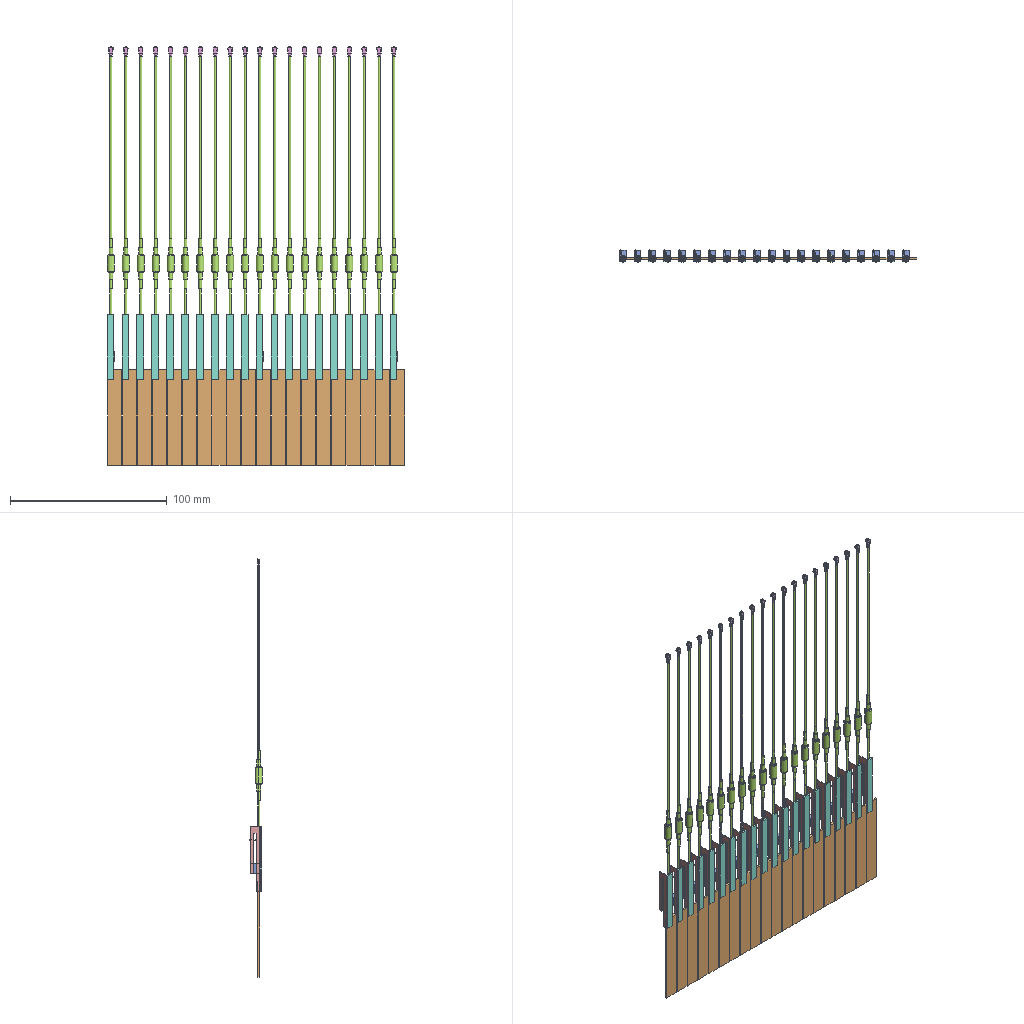Assembly | SolidWorks | 6 different items | 120 placed | box 190 x 8 x 267 mm
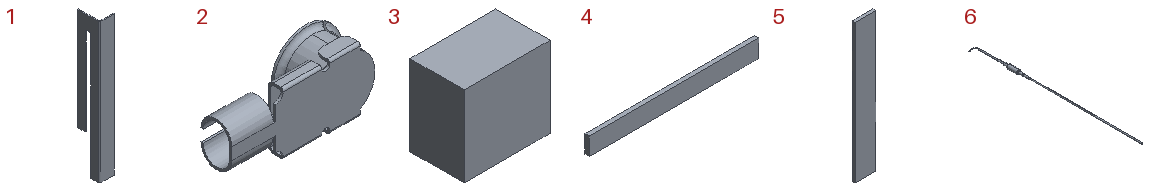Parts list (item | quantity | size | volume | features):
1 | x20 | 4.3 x 6.4 x 41 mm | 101.19 mm3 | features EdgeFlange 1, FlatPattern 1, SMBaseFlange 1, SheetMetal 1
2 | x20 | 6.189 x 1.7 x 2.85 mm | 6.846 mm3 | features ICE 5, EdgeFlange 3, FlatPattern 1, Hem 1, MirrorPattern 1, Revolution 1, SMBaseFlange 1, SheetMetal 1
3 | x20 | 6.5 x 4.1 x 6.1 mm | 162.565 mm3 | features Extrusion 1
4 | x20 | 41 x 1 x 4.3 mm | 176.3 mm3 | features Extrusion 1
5 | x20 | 9 x 1.35 x 61 mm | 702.043 mm3 | features ICE 3, Extrusion 1
6 | x20 | 7.759 x 176.005 x 4.43 mm | 429.128 mm3 | features 3DProfileFeature 2, ICE 2, Revolution 1, Sweep 1
Mates (type | each side: item.copy, entity, surface, feature):
Coordinate | 1.1 select_type:25 | assembly select_type:11
Coincident | 1.1 face plane Base-Flange1 | 3.1 face plane Boss-Extrude1
Coincident | 1.1 face plane Edge-Flange1 | 3.1 face plane Boss-Extrude1 | 2 times
Tangent | 1.1 face plane Base-Flange1 | 6.1 face cylinder Boss-Extrude2 | 2 times
DistanceDim | 1.1 plane | 6.1 plane
DistanceDim | 6.1 face plane Boss-Extrude2 | 1.1 face plane Base-Flange1
Concentric | 6.1 face cylinder Boss-Extrude1 | 2.1 select_type:24
Coincident | 6.1 face plane Boss-Extrude1 | 2.1 face plane Edge-Flange3
Coincident | 1.1 face plane Base-Flange1 | 4.1 face plane Boss-Extrude1 | 3 times
Parallel | 1.1 face plane Edge-Flange1 | 2.1 plane
Coincident | 1.1 face plane Base-Flange1 | 5.1 face plane Boss-Extrude1
DistanceDim | 5.1 face plane Boss-Extrude1 | 3.1 face plane Boss-Extrude1
Coincident | 1.1 face plane Edge-Flange1 | 5.1 face plane Boss-Extrude1